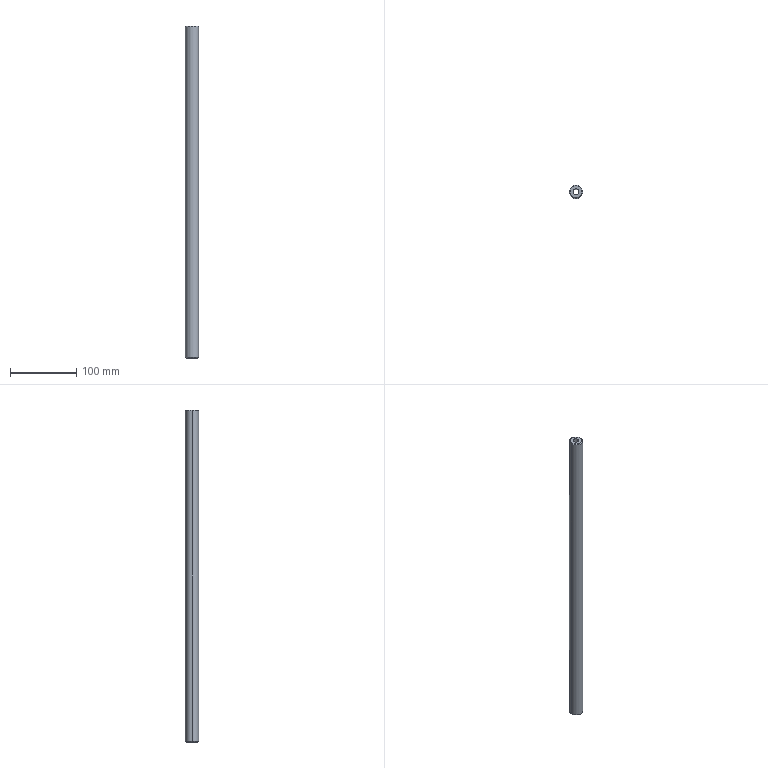Part | Creo | features DATUM PLANE 3, CURVE 2, CHAMFER 1, COORDINATE SYSTEM 1, CUT 1, PROTRUSION 1 | 1 solid | 10 faces | box 20 x 20 x 500 mm | volume 128646 mm3 | cone 4 | cylinder 4 | plane 2 | commonest cylinder face diameters 8.5 x2 20 x2
STEP:
#1=CARTESIAN_POINT('',(0.,0.,0.));
#2=DIRECTION('',(0.,0.,1.));
#3=DIRECTION('',(1.,0.,0.));
#4=AXIS2_PLACEMENT_3D('',#1,#2,#3);
#5=CARTESIAN_POINT('',(9.,0.,0.));
#6=VERTEX_POINT('',#5);
#7=CARTESIAN_POINT('',(-9.,0.,0.));
#8=VERTEX_POINT('',#7);
#9=CARTESIAN_POINT('',(0.,0.,0.));
#10=DIRECTION('',(0.,0.,-1.));
#11=DIRECTION('',(1.,0.,0.));
#12=AXIS2_PLACEMENT_3D('',#9,#10,#11);
#13=CIRCLE('',#12,9.);
#14=EDGE_CURVE('',#6,#8,#13,.T.);
#15=ORIENTED_EDGE('',*,*,#14,.F.);
#16=CARTESIAN_POINT('',(0.,0.,0.));
#17=DIRECTION('',(0.,0.,-1.));
#18=DIRECTION('',(-1.,0.,0.));
#19=AXIS2_PLACEMENT_3D('',#16,#17,#18);
#20=CIRCLE('',#19,9.);
#21=EDGE_CURVE('',#8,#6,#20,.T.);
#22=ORIENTED_EDGE('',*,*,#21,.F.);
#23=EDGE_LOOP('',(#15,#22));
#24=FACE_OUTER_BOUND('',#23,.F.);
#25=CARTESIAN_POINT('',(4.25,0.,0.));
#26=VERTEX_POINT('',#25);
#27=CARTESIAN_POINT('',(-4.25,0.,0.));
#28=VERTEX_POINT('',#27);
#29=CARTESIAN_POINT('',(0.,0.,0.));
#30=DIRECTION('',(0.,0.,1.));
#31=DIRECTION('',(1.,0.,0.));
#32=AXIS2_PLACEMENT_3D('',#29,#30,#31);
#33=CIRCLE('',#32,4.25);
#34=EDGE_CURVE('',#26,#28,#33,.T.);
#35=ORIENTED_EDGE('',*,*,#34,.F.);
#36=CARTESIAN_POINT('',(0.,0.,0.));
#37=DIRECTION('',(0.,0.,1.));
#38=DIRECTION('',(-1.,0.,0.));
#39=AXIS2_PLACEMENT_3D('',#36,#37,#38);
#40=CIRCLE('',#39,4.25);
#41=EDGE_CURVE('',#28,#26,#40,.T.);
#42=ORIENTED_EDGE('',*,*,#41,.F.);
#43=EDGE_LOOP('',(#35,#42));
#44=FACE_BOUND('',#43,.F.);
#45=CARTESIAN_POINT('',(0.,0.,0.));
#46=DIRECTION('',(0.,0.,1.));
#47=DIRECTION('',(1.,0.,0.));
#48=AXIS2_PLACEMENT_3D('',#45,#46,#47);
#49=PLANE('',#48);
#50=ADVANCED_FACE('',(#24,#44),#49,.F.);
#51=ORIENTED_EDGE('',*,*,#14,.T.);
#52=CARTESIAN_POINT('',(-10.,0.,1.));
#53=VERTEX_POINT('',#52);
#54=CARTESIAN_POINT('',(-9.,0.000000377,-0.000000071));
#55=DIRECTION('',(-0.7071,-0.000000044,0.7071));
#56=VECTOR('',#55,1.414);
#57=LINE('',#54,#56);
#58=EDGE_CURVE('',#8,#53,#57,.T.);
#59=ORIENTED_EDGE('',*,*,#58,.T.);
#60=CARTESIAN_POINT('',(10.,0.,1.));
#61=VERTEX_POINT('',#60);
#62=CARTESIAN_POINT('',(0.,0.,1.));
#63=DIRECTION('',(0.,0.,-1.));
#64=DIRECTION('',(1.,0.,0.));
#65=AXIS2_PLACEMENT_3D('',#62,#63,#64);
#66=CIRCLE('',#65,10.);
#67=EDGE_CURVE('',#61,#53,#66,.T.);
#68=ORIENTED_EDGE('',*,*,#67,.F.);
#69=CARTESIAN_POINT('',(9.,-0.000000377,-0.000000071));
#70=DIRECTION('',(0.7071,0.000000044,0.7071));
#71=VECTOR('',#70,1.414);
#72=LINE('',#69,#71);
#73=EDGE_CURVE('',#6,#61,#72,.T.);
#74=ORIENTED_EDGE('',*,*,#73,.F.);
#75=EDGE_LOOP('',(#51,#59,#68,#74));
#76=FACE_OUTER_BOUND('',#75,.F.);
#77=CARTESIAN_POINT('',(0.,0.,0.5));
#78=DIRECTION('',(0.,0.,1.));
#79=DIRECTION('',(0.,-1.,0.));
#80=AXIS2_PLACEMENT_3D('',#77,#78,#79);
#81=CONICAL_SURFACE('',#80,9.5,45.);
#82=ADVANCED_FACE('',(#76),#81,.T.);
#83=ORIENTED_EDGE('',*,*,#21,.T.);
#84=ORIENTED_EDGE('',*,*,#73,.T.);
#85=CARTESIAN_POINT('',(0.,0.,1.));
#86=DIRECTION('',(0.,0.,-1.));
#87=DIRECTION('',(-1.,0.,0.));
#88=AXIS2_PLACEMENT_3D('',#85,#86,#87);
#89=CIRCLE('',#88,10.);
#90=EDGE_CURVE('',#53,#61,#89,.T.);
#91=ORIENTED_EDGE('',*,*,#90,.F.);
#92=ORIENTED_EDGE('',*,*,#58,.F.);
#93=EDGE_LOOP('',(#83,#84,#91,#92));
#94=FACE_OUTER_BOUND('',#93,.F.);
#95=CARTESIAN_POINT('',(0.,0.,0.5));
#96=DIRECTION('',(0.,0.,1.));
#97=DIRECTION('',(0.,-1.,0.));
#98=AXIS2_PLACEMENT_3D('',#95,#96,#97);
#99=CONICAL_SURFACE('',#98,9.5,45.);
#100=ADVANCED_FACE('',(#94),#99,.T.);
#101=ORIENTED_EDGE('',*,*,#90,.T.);
#102=CARTESIAN_POINT('',(10.,0.,499.));
#103=VERTEX_POINT('',#102);
#104=CARTESIAN_POINT('',(10.,-0.000000314,1.));
#105=DIRECTION('',(0.,0.,1.));
#106=VECTOR('',#105,498.);
#107=LINE('',#104,#106);
#108=EDGE_CURVE('',#61,#103,#107,.T.);
#109=ORIENTED_EDGE('',*,*,#108,.T.);
#110=CARTESIAN_POINT('',(-10.,0.,499.));
#111=VERTEX_POINT('',#110);
#112=CARTESIAN_POINT('',(0.,0.,499.));
#113=DIRECTION('',(0.,0.,1.));
#114=DIRECTION('',(1.,0.,0.));
#115=AXIS2_PLACEMENT_3D('',#112,#113,#114);
#116=CIRCLE('',#115,10.);
#117=EDGE_CURVE('',#103,#111,#116,.T.);
#118=ORIENTED_EDGE('',*,*,#117,.T.);
#119=CARTESIAN_POINT('',(-10.,0.000000314,1.));
#120=DIRECTION('',(0.,0.,1.));
#121=VECTOR('',#120,498.);
#122=LINE('',#119,#121);
#123=EDGE_CURVE('',#53,#111,#122,.T.);
#124=ORIENTED_EDGE('',*,*,#123,.F.);
#125=EDGE_LOOP('',(#101,#109,#118,#124));
#126=FACE_OUTER_BOUND('',#125,.F.);
#127=CARTESIAN_POINT('',(0.,0.,0.));
#128=DIRECTION('',(0.,0.,1.));
#129=DIRECTION('',(1.,0.,0.));
#130=AXIS2_PLACEMENT_3D('',#127,#128,#129);
#131=CYLINDRICAL_SURFACE('',#130,10.);
#132=ADVANCED_FACE('',(#126),#131,.T.);
#133=ORIENTED_EDGE('',*,*,#67,.T.);
#134=ORIENTED_EDGE('',*,*,#123,.T.);
#135=CARTESIAN_POINT('',(0.,0.,499.));
#136=DIRECTION('',(0.,0.,1.));
#137=DIRECTION('',(-1.,0.,0.));
#138=AXIS2_PLACEMENT_3D('',#135,#136,#137);
#139=CIRCLE('',#138,10.);
#140=EDGE_CURVE('',#111,#103,#139,.T.);
#141=ORIENTED_EDGE('',*,*,#140,.T.);
#142=ORIENTED_EDGE('',*,*,#108,.F.);
#143=EDGE_LOOP('',(#133,#134,#141,#142));
#144=FACE_OUTER_BOUND('',#143,.F.);
#145=CARTESIAN_POINT('',(0.,0.,0.));
#146=DIRECTION('',(0.,0.,1.));
#147=DIRECTION('',(1.,0.,0.));
#148=AXIS2_PLACEMENT_3D('',#145,#146,#147);
#149=CYLINDRICAL_SURFACE('',#148,10.);
#150=ADVANCED_FACE('',(#144),#149,.T.);
#151=CARTESIAN_POINT('',(-9.,0.,500.));
#152=VERTEX_POINT('',#151);
#153=CARTESIAN_POINT('',(9.,0.,500.));
#154=VERTEX_POINT('',#153);
#155=CARTESIAN_POINT('',(0.,0.,500.));
#156=DIRECTION('',(0.,0.,1.));
#157=DIRECTION('',(-1.,0.,0.));
#158=AXIS2_PLACEMENT_3D('',#155,#156,#157);
#159=CIRCLE('',#158,9.);
#160=EDGE_CURVE('',#152,#154,#159,.T.);
#161=ORIENTED_EDGE('',*,*,#160,.T.);
#162=CARTESIAN_POINT('',(9.,-0.000000377,500.));
#163=DIRECTION('',(0.7071,0.000000044,-0.7071));
#164=VECTOR('',#163,1.414);
#165=LINE('',#162,#164);
#166=EDGE_CURVE('',#154,#103,#165,.T.);
#167=ORIENTED_EDGE('',*,*,#166,.T.);
#168=ORIENTED_EDGE('',*,*,#140,.F.);
#169=CARTESIAN_POINT('',(-9.,0.000000377,500.));
#170=DIRECTION('',(-0.7071,-0.000000044,-0.7071));
#171=VECTOR('',#170,1.414);
#172=LINE('',#169,#171);
#173=EDGE_CURVE('',#152,#111,#172,.T.);
#174=ORIENTED_EDGE('',*,*,#173,.F.);
#175=EDGE_LOOP('',(#161,#167,#168,#174));
#176=FACE_OUTER_BOUND('',#175,.F.);
#177=CARTESIAN_POINT('',(0.,0.,499.5));
#178=DIRECTION('',(0.,0.,-1.));
#179=DIRECTION('',(0.,-1.,0.));
#180=AXIS2_PLACEMENT_3D('',#177,#178,#179);
#181=CONICAL_SURFACE('',#180,9.5,45.);
#182=ADVANCED_FACE('',(#176),#181,.T.);
#183=ORIENTED_EDGE('',*,*,#160,.F.);
#184=CARTESIAN_POINT('',(0.,0.,500.));
#185=DIRECTION('',(0.,0.,1.));
#186=DIRECTION('',(1.,0.,0.));
#187=AXIS2_PLACEMENT_3D('',#184,#185,#186);
#188=CIRCLE('',#187,9.);
#189=EDGE_CURVE('',#154,#152,#188,.T.);
#190=ORIENTED_EDGE('',*,*,#189,.F.);
#191=EDGE_LOOP('',(#183,#190));
#192=FACE_OUTER_BOUND('',#191,.F.);
#193=CARTESIAN_POINT('',(4.25,0.,500.));
#194=VERTEX_POINT('',#193);
#195=CARTESIAN_POINT('',(-4.25,0.,500.));
#196=VERTEX_POINT('',#195);
#197=CARTESIAN_POINT('',(0.,0.,500.));
#198=DIRECTION('',(0.,0.,1.));
#199=DIRECTION('',(1.,0.,0.));
#200=AXIS2_PLACEMENT_3D('',#197,#198,#199);
#201=CIRCLE('',#200,4.25);
#202=EDGE_CURVE('',#194,#196,#201,.T.);
#203=ORIENTED_EDGE('',*,*,#202,.T.);
#204=CARTESIAN_POINT('',(0.,0.,500.));
#205=DIRECTION('',(0.,0.,1.));
#206=DIRECTION('',(-1.,0.,0.));
#207=AXIS2_PLACEMENT_3D('',#204,#205,#206);
#208=CIRCLE('',#207,4.25);
#209=EDGE_CURVE('',#196,#194,#208,.T.);
#210=ORIENTED_EDGE('',*,*,#209,.T.);
#211=EDGE_LOOP('',(#203,#210));
#212=FACE_BOUND('',#211,.F.);
#213=CARTESIAN_POINT('',(0.,0.,500.));
#214=DIRECTION('',(0.,0.,1.));
#215=DIRECTION('',(1.,0.,0.));
#216=AXIS2_PLACEMENT_3D('',#213,#214,#215);
#217=PLANE('',#216);
#218=ADVANCED_FACE('',(#192,#212),#217,.T.);
#219=ORIENTED_EDGE('',*,*,#189,.T.);
#220=ORIENTED_EDGE('',*,*,#173,.T.);
#221=ORIENTED_EDGE('',*,*,#117,.F.);
#222=ORIENTED_EDGE('',*,*,#166,.F.);
#223=EDGE_LOOP('',(#219,#220,#221,#222));
#224=FACE_OUTER_BOUND('',#223,.F.);
#225=CARTESIAN_POINT('',(0.,0.,499.5));
#226=DIRECTION('',(0.,0.,-1.));
#227=DIRECTION('',(0.,-1.,0.));
#228=AXIS2_PLACEMENT_3D('',#225,#226,#227);
#229=CONICAL_SURFACE('',#228,9.5,45.);
#230=ADVANCED_FACE('',(#224),#229,.T.);
#231=ORIENTED_EDGE('',*,*,#202,.F.);
#232=CARTESIAN_POINT('',(4.25,0.,500.));
#233=DIRECTION('',(0.,0.,-1.));
#234=VECTOR('',#233,500.);
#235=LINE('',#232,#234);
#236=EDGE_CURVE('',#194,#26,#235,.T.);
#237=ORIENTED_EDGE('',*,*,#236,.T.);
#238=ORIENTED_EDGE('',*,*,#34,.T.);
#239=CARTESIAN_POINT('',(-4.25,0.,500.));
#240=DIRECTION('',(0.,0.,-1.));
#241=VECTOR('',#240,500.);
#242=LINE('',#239,#241);
#243=EDGE_CURVE('',#196,#28,#242,.T.);
#244=ORIENTED_EDGE('',*,*,#243,.F.);
#245=EDGE_LOOP('',(#231,#237,#238,#244));
#246=FACE_OUTER_BOUND('',#245,.F.);
#247=CARTESIAN_POINT('',(0.,0.,500.));
#248=DIRECTION('',(0.,0.,1.));
#249=DIRECTION('',(1.,0.,0.));
#250=AXIS2_PLACEMENT_3D('',#247,#248,#249);
#251=CYLINDRICAL_SURFACE('',#250,4.25);
#252=ADVANCED_FACE('',(#246),#251,.F.);
#253=ORIENTED_EDGE('',*,*,#209,.F.);
#254=ORIENTED_EDGE('',*,*,#243,.T.);
#255=ORIENTED_EDGE('',*,*,#41,.T.);
#256=ORIENTED_EDGE('',*,*,#236,.F.);
#257=EDGE_LOOP('',(#253,#254,#255,#256));
#258=FACE_OUTER_BOUND('',#257,.F.);
#259=CARTESIAN_POINT('',(0.,0.,500.));
#260=DIRECTION('',(0.,0.,1.));
#261=DIRECTION('',(1.,0.,0.));
#262=AXIS2_PLACEMENT_3D('',#259,#260,#261);
#263=CYLINDRICAL_SURFACE('',#262,4.25);
#264=ADVANCED_FACE('',(#258),#263,.F.);
#265=CLOSED_SHELL('',(#50,#82,#100,#132,#150,#182,#218,#230,#252,#264));
#266=MANIFOLD_SOLID_BREP('',#265);
#267=(LENGTH_UNIT()NAMED_UNIT(*)SI_UNIT(.MILLI.,.METRE.));
#268=UNCERTAINTY_MEASURE_WITH_UNIT(LENGTH_MEASURE(0.05008),#267,'','');
#269=(NAMED_UNIT(*)PLANE_ANGLE_UNIT()SI_UNIT($,.RADIAN.));
#270=PLANE_ANGLE_MEASURE_WITH_UNIT(PLANE_ANGLE_MEASURE(0.01745),#269);
#271=(CONVERSION_BASED_UNIT('DEGREE',#270)NAMED_UNIT(*)PLANE_ANGLE_UNIT());
#272=(NAMED_UNIT(*)SI_UNIT($,.STERADIAN.)SOLID_ANGLE_UNIT());
#273=(GEOMETRIC_REPRESENTATION_CONTEXT(3)GLOBAL_UNCERTAINTY_ASSIGNED_CONTEXT((#268))GLOBAL_UNIT_ASSIGNED_CONTEXT((#267,#271,#272))REPRESENTATION_CONTEXT('',''));
#274=ADVANCED_BREP_SHAPE_REPRESENTATION('',(#4,#266),#273);